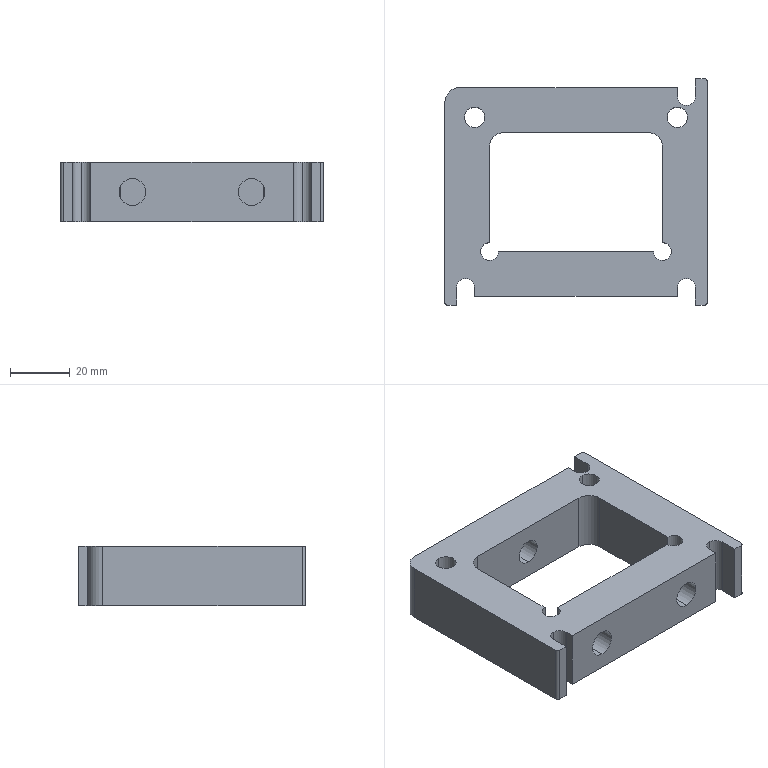Part | 1 solid | 45 faces | box 88 x 76 x 20 mm | volume 70626 mm3 | cylinder 26 | plane 19 | commonest cylinder face diameters 6 x10 6.8 x4 9 x4 2 x3 10 x3 8.5 x2
STEP:
#1=CARTESIAN_POINT('',(37.,29.,0.));
#2=VERTEX_POINT('',#1);
#3=CARTESIAN_POINT('',(34.,32.,0.));
#4=VERTEX_POINT('',#3);
#5=CARTESIAN_POINT('',(37.,32.,0.));
#6=DIRECTION('',(0.,0.,-1.));
#7=DIRECTION('',(0.,-1.,0.));
#8=AXIS2_PLACEMENT_3D('',#5,#6,#7);
#9=CIRCLE('',#8,3.);
#10=EDGE_CURVE('',#2,#4,#9,.T.);
#11=ORIENTED_EDGE('',*,*,#10,.F.);
#12=CARTESIAN_POINT('',(37.,29.,-20.));
#13=VERTEX_POINT('',#12);
#14=CARTESIAN_POINT('',(37.,29.,0.));
#15=DIRECTION('',(0.,0.,-1.));
#16=VECTOR('',#15,1000.);
#17=LINE('',#14,#16);
#18=EDGE_CURVE('',#2,#13,#17,.T.);
#19=ORIENTED_EDGE('',*,*,#18,.T.);
#20=CARTESIAN_POINT('',(34.,32.,-20.));
#21=VERTEX_POINT('',#20);
#22=CARTESIAN_POINT('',(37.,32.,-20.));
#23=DIRECTION('',(0.,0.,-1.));
#24=DIRECTION('',(0.,-1.,0.));
#25=AXIS2_PLACEMENT_3D('',#22,#23,#24);
#26=CIRCLE('',#25,3.);
#27=EDGE_CURVE('',#13,#21,#26,.T.);
#28=ORIENTED_EDGE('',*,*,#27,.T.);
#29=CARTESIAN_POINT('',(34.,32.,0.));
#30=DIRECTION('',(0.,0.,-1.));
#31=VECTOR('',#30,1000.);
#32=LINE('',#29,#31);
#33=EDGE_CURVE('',#4,#21,#32,.T.);
#34=ORIENTED_EDGE('',*,*,#33,.F.);
#35=EDGE_LOOP('',(#11,#19,#28,#34));
#36=FACE_BOUND('',#35,.T.);
#37=CARTESIAN_POINT('',(37.,32.,0.));
#38=DIRECTION('',(0.,0.,-1.));
#39=DIRECTION('',(0.,1.,0.));
#40=AXIS2_PLACEMENT_3D('',#37,#38,#39);
#41=CYLINDRICAL_SURFACE('',#40,3.);
#42=ADVANCED_FACE('',(#36),#41,.F.);
#43=CARTESIAN_POINT('',(-34.,21.6,0.));
#44=VERTEX_POINT('',#43);
#45=CARTESIAN_POINT('',(-34.,28.4,0.));
#46=VERTEX_POINT('',#45);
#47=CARTESIAN_POINT('',(-34.,25.,0.));
#48=DIRECTION('',(0.,0.,1.));
#49=DIRECTION('',(0.,1.,0.));
#50=AXIS2_PLACEMENT_3D('',#47,#48,#49);
#51=CIRCLE('',#50,3.4);
#52=EDGE_CURVE('',#44,#46,#51,.T.);
#53=ORIENTED_EDGE('',*,*,#52,.T.);
#54=CARTESIAN_POINT('',(-34.,28.4,-20.));
#55=VERTEX_POINT('',#54);
#56=CARTESIAN_POINT('',(-34.,28.4,-20.));
#57=DIRECTION('',(0.,0.,-1.));
#58=VECTOR('',#57,1000.);
#59=LINE('',#56,#58);
#60=EDGE_CURVE('',#55,#46,#59,.F.);
#61=ORIENTED_EDGE('',*,*,#60,.F.);
#62=CARTESIAN_POINT('',(-34.,21.6,-20.));
#63=VERTEX_POINT('',#62);
#64=CARTESIAN_POINT('',(-34.,25.,-20.));
#65=DIRECTION('',(0.,0.,-1.));
#66=DIRECTION('',(0.,-1.,0.));
#67=AXIS2_PLACEMENT_3D('',#64,#65,#66);
#68=CIRCLE('',#67,3.4);
#69=EDGE_CURVE('',#55,#63,#68,.T.);
#70=ORIENTED_EDGE('',*,*,#69,.T.);
#71=CARTESIAN_POINT('',(-34.,21.6,-20.));
#72=DIRECTION('',(0.,0.,-1.));
#73=VECTOR('',#72,1000.);
#74=LINE('',#71,#73);
#75=EDGE_CURVE('',#63,#44,#74,.F.);
#76=ORIENTED_EDGE('',*,*,#75,.T.);
#77=EDGE_LOOP('',(#53,#61,#70,#76));
#78=FACE_BOUND('',#77,.T.);
#79=CARTESIAN_POINT('',(-34.,25.,-20.));
#80=DIRECTION('',(0.,0.,-1.));
#81=DIRECTION('',(0.,1.,0.));
#82=AXIS2_PLACEMENT_3D('',#79,#80,#81);
#83=CYLINDRICAL_SURFACE('',#82,3.4);
#84=ADVANCED_FACE('',(#78),#83,.F.);
#85=CARTESIAN_POINT('',(34.,21.6,0.));
#86=VERTEX_POINT('',#85);
#87=CARTESIAN_POINT('',(34.,28.4,0.));
#88=VERTEX_POINT('',#87);
#89=CARTESIAN_POINT('',(34.,25.,0.));
#90=DIRECTION('',(0.,0.,1.));
#91=DIRECTION('',(0.,1.,0.));
#92=AXIS2_PLACEMENT_3D('',#89,#90,#91);
#93=CIRCLE('',#92,3.4);
#94=EDGE_CURVE('',#86,#88,#93,.T.);
#95=ORIENTED_EDGE('',*,*,#94,.T.);
#96=CARTESIAN_POINT('',(34.,28.4,-20.));
#97=VERTEX_POINT('',#96);
#98=CARTESIAN_POINT('',(34.,28.4,-20.));
#99=DIRECTION('',(0.,0.,-1.));
#100=VECTOR('',#99,1000.);
#101=LINE('',#98,#100);
#102=EDGE_CURVE('',#97,#88,#101,.F.);
#103=ORIENTED_EDGE('',*,*,#102,.F.);
#104=CARTESIAN_POINT('',(34.,21.6,-20.));
#105=VERTEX_POINT('',#104);
#106=CARTESIAN_POINT('',(34.,25.,-20.));
#107=DIRECTION('',(0.,0.,-1.));
#108=DIRECTION('',(0.,-1.,0.));
#109=AXIS2_PLACEMENT_3D('',#106,#107,#108);
#110=CIRCLE('',#109,3.4);
#111=EDGE_CURVE('',#97,#105,#110,.T.);
#112=ORIENTED_EDGE('',*,*,#111,.T.);
#113=CARTESIAN_POINT('',(34.,21.6,-20.));
#114=DIRECTION('',(0.,0.,-1.));
#115=VECTOR('',#114,1000.);
#116=LINE('',#113,#115);
#117=EDGE_CURVE('',#105,#86,#116,.F.);
#118=ORIENTED_EDGE('',*,*,#117,.T.);
#119=EDGE_LOOP('',(#95,#103,#112,#118));
#120=FACE_BOUND('',#119,.T.);
#121=CARTESIAN_POINT('',(34.,25.,-20.));
#122=DIRECTION('',(0.,0.,-1.));
#123=DIRECTION('',(0.,1.,0.));
#124=AXIS2_PLACEMENT_3D('',#121,#122,#123);
#125=CYLINDRICAL_SURFACE('',#124,3.4);
#126=ADVANCED_FACE('',(#120),#125,.F.);
#127=CARTESIAN_POINT('',(29.,-23.,0.));
#128=VERTEX_POINT('',#127);
#129=CARTESIAN_POINT('',(26.,-20.,0.));
#130=VERTEX_POINT('',#129);
#131=CARTESIAN_POINT('',(29.,-20.,0.));
#132=DIRECTION('',(0.,0.,-1.));
#133=DIRECTION('',(0.,-1.,0.));
#134=AXIS2_PLACEMENT_3D('',#131,#132,#133);
#135=CIRCLE('',#134,3.);
#136=EDGE_CURVE('',#128,#130,#135,.T.);
#137=ORIENTED_EDGE('',*,*,#136,.F.);
#138=CARTESIAN_POINT('',(29.,-23.,-20.));
#139=VERTEX_POINT('',#138);
#140=CARTESIAN_POINT('',(29.,-23.,0.));
#141=DIRECTION('',(0.,0.,-1.));
#142=VECTOR('',#141,1000.);
#143=LINE('',#140,#142);
#144=EDGE_CURVE('',#128,#139,#143,.T.);
#145=ORIENTED_EDGE('',*,*,#144,.T.);
#146=CARTESIAN_POINT('',(26.,-20.,-20.));
#147=VERTEX_POINT('',#146);
#148=CARTESIAN_POINT('',(29.,-20.,-20.));
#149=DIRECTION('',(0.,0.,-1.));
#150=DIRECTION('',(0.,-1.,0.));
#151=AXIS2_PLACEMENT_3D('',#148,#149,#150);
#152=CIRCLE('',#151,3.);
#153=EDGE_CURVE('',#139,#147,#152,.T.);
#154=ORIENTED_EDGE('',*,*,#153,.T.);
#155=CARTESIAN_POINT('',(26.,-20.,0.));
#156=DIRECTION('',(0.,0.,-1.));
#157=VECTOR('',#156,1000.);
#158=LINE('',#155,#157);
#159=EDGE_CURVE('',#130,#147,#158,.T.);
#160=ORIENTED_EDGE('',*,*,#159,.F.);
#161=EDGE_LOOP('',(#137,#145,#154,#160));
#162=FACE_BOUND('',#161,.T.);
#163=CARTESIAN_POINT('',(29.,-20.,0.));
#164=DIRECTION('',(0.,0.,-1.));
#165=DIRECTION('',(0.,1.,0.));
#166=AXIS2_PLACEMENT_3D('',#163,#164,#165);
#167=CYLINDRICAL_SURFACE('',#166,3.);
#168=ADVANCED_FACE('',(#162),#167,.F.);
#169=CARTESIAN_POINT('',(-29.,-23.,0.));
#170=VERTEX_POINT('',#169);
#171=CARTESIAN_POINT('',(-29.,-17.,0.));
#172=VERTEX_POINT('',#171);
#173=CARTESIAN_POINT('',(-29.,-20.,0.));
#174=DIRECTION('',(0.,0.,-1.));
#175=DIRECTION('',(0.,-1.,0.));
#176=AXIS2_PLACEMENT_3D('',#173,#174,#175);
#177=CIRCLE('',#176,3.);
#178=EDGE_CURVE('',#170,#172,#177,.T.);
#179=ORIENTED_EDGE('',*,*,#178,.F.);
#180=CARTESIAN_POINT('',(-29.,-23.,-20.));
#181=VERTEX_POINT('',#180);
#182=CARTESIAN_POINT('',(-29.,-23.,0.));
#183=DIRECTION('',(0.,0.,-1.));
#184=VECTOR('',#183,1000.);
#185=LINE('',#182,#184);
#186=EDGE_CURVE('',#170,#181,#185,.T.);
#187=ORIENTED_EDGE('',*,*,#186,.T.);
#188=CARTESIAN_POINT('',(-29.,-17.,-20.));
#189=VERTEX_POINT('',#188);
#190=CARTESIAN_POINT('',(-29.,-20.,-20.));
#191=DIRECTION('',(0.,0.,-1.));
#192=DIRECTION('',(0.,-1.,0.));
#193=AXIS2_PLACEMENT_3D('',#190,#191,#192);
#194=CIRCLE('',#193,3.);
#195=EDGE_CURVE('',#181,#189,#194,.T.);
#196=ORIENTED_EDGE('',*,*,#195,.T.);
#197=CARTESIAN_POINT('',(-29.,-17.,0.));
#198=DIRECTION('',(0.,0.,-1.));
#199=VECTOR('',#198,1000.);
#200=LINE('',#197,#199);
#201=EDGE_CURVE('',#172,#189,#200,.T.);
#202=ORIENTED_EDGE('',*,*,#201,.F.);
#203=EDGE_LOOP('',(#179,#187,#196,#202));
#204=FACE_BOUND('',#203,.T.);
#205=CARTESIAN_POINT('',(-29.,-20.,0.));
#206=DIRECTION('',(0.,0.,-1.));
#207=DIRECTION('',(0.,1.,0.));
#208=AXIS2_PLACEMENT_3D('',#205,#206,#207);
#209=CYLINDRICAL_SURFACE('',#208,3.);
#210=ADVANCED_FACE('',(#204),#209,.F.);
#211=CARTESIAN_POINT('',(20.,-20.,-5.5));
#212=VERTEX_POINT('',#211);
#213=CARTESIAN_POINT('',(20.,-20.,-14.5));
#214=VERTEX_POINT('',#213);
#215=CARTESIAN_POINT('',(20.,-20.,-10.));
#216=DIRECTION('',(0.,1.,0.));
#217=DIRECTION('',(0.,0.,1.));
#218=AXIS2_PLACEMENT_3D('',#215,#216,#217);
#219=CIRCLE('',#218,4.5);
#220=EDGE_CURVE('',#212,#214,#219,.T.);
#221=ORIENTED_EDGE('',*,*,#220,.T.);
#222=CARTESIAN_POINT('',(20.,-35.,-14.5));
#223=VERTEX_POINT('',#222);
#224=CARTESIAN_POINT('',(20.,15.,-14.5));
#225=DIRECTION('',(0.,-1.,0.));
#226=VECTOR('',#225,1000.);
#227=LINE('',#224,#226);
#228=EDGE_CURVE('',#223,#214,#227,.F.);
#229=ORIENTED_EDGE('',*,*,#228,.F.);
#230=CARTESIAN_POINT('',(20.,-35.,-5.5));
#231=VERTEX_POINT('',#230);
#232=CARTESIAN_POINT('',(20.,-35.,-10.));
#233=DIRECTION('',(0.,1.,0.));
#234=DIRECTION('',(0.,0.,1.));
#235=AXIS2_PLACEMENT_3D('',#232,#233,#234);
#236=CIRCLE('',#235,4.5);
#237=EDGE_CURVE('',#231,#223,#236,.T.);
#238=ORIENTED_EDGE('',*,*,#237,.F.);
#239=CARTESIAN_POINT('',(20.,15.,-5.5));
#240=DIRECTION('',(0.,-1.,0.));
#241=VECTOR('',#240,1000.);
#242=LINE('',#239,#241);
#243=EDGE_CURVE('',#231,#212,#242,.F.);
#244=ORIENTED_EDGE('',*,*,#243,.T.);
#245=EDGE_LOOP('',(#221,#229,#238,#244));
#246=FACE_BOUND('',#245,.T.);
#247=CARTESIAN_POINT('',(20.,15.,-10.));
#248=DIRECTION('',(0.,-1.,0.));
#249=DIRECTION('',(0.,0.,-1.));
#250=AXIS2_PLACEMENT_3D('',#247,#248,#249);
#251=CYLINDRICAL_SURFACE('',#250,4.5);
#252=ADVANCED_FACE('',(#246),#251,.F.);
#253=CARTESIAN_POINT('',(-20.,-20.,-14.5));
#254=VERTEX_POINT('',#253);
#255=CARTESIAN_POINT('',(-20.,-20.,-5.5));
#256=VERTEX_POINT('',#255);
#257=CARTESIAN_POINT('',(-20.,-20.,-10.));
#258=DIRECTION('',(0.,-1.,0.));
#259=DIRECTION('',(0.,0.,1.));
#260=AXIS2_PLACEMENT_3D('',#257,#258,#259);
#261=CIRCLE('',#260,4.5);
#262=EDGE_CURVE('',#254,#256,#261,.T.);
#263=ORIENTED_EDGE('',*,*,#262,.F.);
#264=CARTESIAN_POINT('',(-20.,-35.,-14.5));
#265=VERTEX_POINT('',#264);
#266=CARTESIAN_POINT('',(-20.,15.,-14.5));
#267=DIRECTION('',(0.,-1.,0.));
#268=VECTOR('',#267,1000.);
#269=LINE('',#266,#268);
#270=EDGE_CURVE('',#265,#254,#269,.F.);
#271=ORIENTED_EDGE('',*,*,#270,.F.);
#272=CARTESIAN_POINT('',(-20.,-35.,-5.5));
#273=VERTEX_POINT('',#272);
#274=CARTESIAN_POINT('',(-20.,-35.,-10.));
#275=DIRECTION('',(0.,-1.,0.));
#276=DIRECTION('',(0.,0.,1.));
#277=AXIS2_PLACEMENT_3D('',#274,#275,#276);
#278=CIRCLE('',#277,4.5);
#279=EDGE_CURVE('',#265,#273,#278,.T.);
#280=ORIENTED_EDGE('',*,*,#279,.T.);
#281=CARTESIAN_POINT('',(-20.,15.,-5.5));
#282=DIRECTION('',(0.,-1.,0.));
#283=VECTOR('',#282,1000.);
#284=LINE('',#281,#283);
#285=EDGE_CURVE('',#273,#256,#284,.F.);
#286=ORIENTED_EDGE('',*,*,#285,.T.);
#287=EDGE_LOOP('',(#263,#271,#280,#286));
#288=FACE_BOUND('',#287,.T.);
#289=CARTESIAN_POINT('',(-20.,15.,-10.));
#290=DIRECTION('',(0.,-1.,0.));
#291=DIRECTION('',(0.,0.,-1.));
#292=AXIS2_PLACEMENT_3D('',#289,#290,#291);
#293=CYLINDRICAL_SURFACE('',#292,4.5);
#294=ADVANCED_FACE('',(#288),#293,.F.);
#295=CARTESIAN_POINT('',(0.,20.,-5.75));
#296=VERTEX_POINT('',#295);
#297=CARTESIAN_POINT('',(0.,20.,-14.25));
#298=VERTEX_POINT('',#297);
#299=CARTESIAN_POINT('',(0.,20.,-10.));
#300=DIRECTION('',(0.,1.,0.));
#301=DIRECTION('',(0.,0.,-1.));
#302=AXIS2_PLACEMENT_3D('',#299,#300,#301);
#303=CIRCLE('',#302,4.25);
#304=EDGE_CURVE('',#296,#298,#303,.T.);
#305=ORIENTED_EDGE('',*,*,#304,.F.);
#306=CARTESIAN_POINT('',(0.,35.,-5.75));
#307=VERTEX_POINT('',#306);
#308=CARTESIAN_POINT('',(0.,35.,-5.75));
#309=DIRECTION('',(0.,1.,0.));
#310=VECTOR('',#309,1000.);
#311=LINE('',#308,#310);
#312=EDGE_CURVE('',#307,#296,#311,.F.);
#313=ORIENTED_EDGE('',*,*,#312,.F.);
#314=CARTESIAN_POINT('',(0.,35.,-14.25));
#315=VERTEX_POINT('',#314);
#316=CARTESIAN_POINT('',(0.,35.,-10.));
#317=DIRECTION('',(0.,1.,0.));
#318=DIRECTION('',(0.,0.,-1.));
#319=AXIS2_PLACEMENT_3D('',#316,#317,#318);
#320=CIRCLE('',#319,4.25);
#321=EDGE_CURVE('',#307,#315,#320,.T.);
#322=ORIENTED_EDGE('',*,*,#321,.T.);
#323=CARTESIAN_POINT('',(0.,35.,-14.25));
#324=DIRECTION('',(0.,1.,0.));
#325=VECTOR('',#324,1000.);
#326=LINE('',#323,#325);
#327=EDGE_CURVE('',#315,#298,#326,.F.);
#328=ORIENTED_EDGE('',*,*,#327,.T.);
#329=EDGE_LOOP('',(#305,#313,#322,#328));
#330=FACE_BOUND('',#329,.T.);
#331=CARTESIAN_POINT('',(0.,35.,-10.));
#332=DIRECTION('',(0.,1.,0.));
#333=DIRECTION('',(0.,0.,1.));
#334=AXIS2_PLACEMENT_3D('',#331,#332,#333);
#335=CYLINDRICAL_SURFACE('',#334,4.25);
#336=ADVANCED_FACE('',(#330),#335,.F.);
#337=CARTESIAN_POINT('',(-29.,15.,-20.));
#338=VERTEX_POINT('',#337);
#339=CARTESIAN_POINT('',(-29.,20.,-20.));
#340=DIRECTION('',(0.,1.,0.));
#341=VECTOR('',#340,1000.);
#342=LINE('',#339,#341);
#343=EDGE_CURVE('',#189,#338,#342,.T.);
#344=ORIENTED_EDGE('',*,*,#343,.F.);
#345=ORIENTED_EDGE('',*,*,#195,.F.);
#346=CARTESIAN_POINT('',(-26.,-20.,-20.));
#347=VERTEX_POINT('',#346);
#348=CARTESIAN_POINT('',(-29.,-20.,-20.));
#349=DIRECTION('',(0.,0.,-1.));
#350=DIRECTION('',(0.,-1.,0.));
#351=AXIS2_PLACEMENT_3D('',#348,#349,#350);
#352=CIRCLE('',#351,3.);
#353=EDGE_CURVE('',#347,#181,#352,.T.);
#354=ORIENTED_EDGE('',*,*,#353,.F.);
#355=CARTESIAN_POINT('',(29.,-20.,-20.));
#356=DIRECTION('',(-1.,0.,0.));
#357=VECTOR('',#356,1000.);
#358=LINE('',#355,#357);
#359=EDGE_CURVE('',#147,#347,#358,.T.);
#360=ORIENTED_EDGE('',*,*,#359,.F.);
#361=ORIENTED_EDGE('',*,*,#153,.F.);
#362=CARTESIAN_POINT('',(29.,-17.,-20.));
#363=VERTEX_POINT('',#362);
#364=CARTESIAN_POINT('',(29.,-20.,-20.));
#365=DIRECTION('',(0.,0.,-1.));
#366=DIRECTION('',(0.,-1.,0.));
#367=AXIS2_PLACEMENT_3D('',#364,#365,#366);
#368=CIRCLE('',#367,3.);
#369=EDGE_CURVE('',#363,#139,#368,.T.);
#370=ORIENTED_EDGE('',*,*,#369,.F.);
#371=CARTESIAN_POINT('',(29.,15.,-20.));
#372=VERTEX_POINT('',#371);
#373=CARTESIAN_POINT('',(29.,20.,-20.));
#374=DIRECTION('',(0.,-1.,0.));
#375=VECTOR('',#374,1000.);
#376=LINE('',#373,#375);
#377=EDGE_CURVE('',#372,#363,#376,.T.);
#378=ORIENTED_EDGE('',*,*,#377,.F.);
#379=CARTESIAN_POINT('',(24.,20.,-20.));
#380=VERTEX_POINT('',#379);
#381=CARTESIAN_POINT('',(24.,15.,-20.));
#382=DIRECTION('',(0.,0.,1.));
#383=DIRECTION('',(0.,1.,0.));
#384=AXIS2_PLACEMENT_3D('',#381,#382,#383);
#385=CIRCLE('',#384,5.);
#386=EDGE_CURVE('',#372,#380,#385,.T.);
#387=ORIENTED_EDGE('',*,*,#386,.T.);
#388=CARTESIAN_POINT('',(-24.,20.,-20.));
#389=VERTEX_POINT('',#388);
#390=CARTESIAN_POINT('',(29.,20.,-20.));
#391=DIRECTION('',(1.,0.,0.));
#392=VECTOR('',#391,1000.);
#393=LINE('',#390,#392);
#394=EDGE_CURVE('',#389,#380,#393,.T.);
#395=ORIENTED_EDGE('',*,*,#394,.F.);
#396=CARTESIAN_POINT('',(-24.,15.,-20.));
#397=DIRECTION('',(0.,0.,1.));
#398=DIRECTION('',(0.,1.,0.));
#399=AXIS2_PLACEMENT_3D('',#396,#397,#398);
#400=CIRCLE('',#399,5.);
#401=EDGE_CURVE('',#389,#338,#400,.T.);
#402=ORIENTED_EDGE('',*,*,#401,.T.);
#403=EDGE_LOOP('',(#344,#345,#354,#360,#361,#370,#378,#387,#395,#402));
#404=FACE_BOUND('',#403,.T.);
#405=CARTESIAN_POINT('',(34.,25.,-20.));
#406=DIRECTION('',(0.,0.,-1.));
#407=DIRECTION('',(0.,-1.,0.));
#408=AXIS2_PLACEMENT_3D('',#405,#406,#407);
#409=CIRCLE('',#408,3.4);
#410=EDGE_CURVE('',#105,#97,#409,.T.);
#411=ORIENTED_EDGE('',*,*,#410,.F.);
#412=ORIENTED_EDGE('',*,*,#111,.F.);
#413=EDGE_LOOP('',(#411,#412));
#414=FACE_BOUND('',#413,.T.);
#415=CARTESIAN_POINT('',(-34.,25.,-20.));
#416=DIRECTION('',(0.,0.,-1.));
#417=DIRECTION('',(0.,-1.,0.));
#418=AXIS2_PLACEMENT_3D('',#415,#416,#417);
#419=CIRCLE('',#418,3.4);
#420=EDGE_CURVE('',#63,#55,#419,.T.);
#421=ORIENTED_EDGE('',*,*,#420,.F.);
#422=ORIENTED_EDGE('',*,*,#69,.F.);
#423=EDGE_LOOP('',(#421,#422));
#424=FACE_BOUND('',#423,.T.);
#425=CARTESIAN_POINT('',(-40.,-38.,-20.));
#426=VERTEX_POINT('',#425);
#427=CARTESIAN_POINT('',(-43.,-38.,-20.));
#428=VERTEX_POINT('',#427);
#429=CARTESIAN_POINT('',(44.,-38.,-20.));
#430=DIRECTION('',(-1.,0.,0.));
#431=VECTOR('',#430,1000.);
#432=LINE('',#429,#431);
#433=EDGE_CURVE('',#426,#428,#432,.T.);
#434=ORIENTED_EDGE('',*,*,#433,.T.);
#435=CARTESIAN_POINT('',(-44.,-37.,-20.));
#436=VERTEX_POINT('',#435);
#437=CARTESIAN_POINT('',(-43.,-37.,-20.));
#438=DIRECTION('',(0.,0.,-1.));
#439=DIRECTION('',(0.,1.,0.));
#440=AXIS2_PLACEMENT_3D('',#437,#438,#439);
#441=CIRCLE('',#440,1.);
#442=EDGE_CURVE('',#428,#436,#441,.T.);
#443=ORIENTED_EDGE('',*,*,#442,.T.);
#444=CARTESIAN_POINT('',(-44.,30.,-20.));
#445=VERTEX_POINT('',#444);
#446=CARTESIAN_POINT('',(-44.,38.,-20.));
#447=DIRECTION('',(0.,1.,0.));
#448=VECTOR('',#447,1000.);
#449=LINE('',#446,#448);
#450=EDGE_CURVE('',#436,#445,#449,.T.);
#451=ORIENTED_EDGE('',*,*,#450,.T.);
#452=CARTESIAN_POINT('',(-39.,35.,-20.));
#453=VERTEX_POINT('',#452);
#454=CARTESIAN_POINT('',(-39.,30.,-20.));
#455=DIRECTION('',(0.,0.,-1.));
#456=DIRECTION('',(0.,1.,0.));
#457=AXIS2_PLACEMENT_3D('',#454,#455,#456);
#458=CIRCLE('',#457,5.);
#459=EDGE_CURVE('',#445,#453,#458,.T.);
#460=ORIENTED_EDGE('',*,*,#459,.T.);
#461=CARTESIAN_POINT('',(34.,35.,-20.));
#462=VERTEX_POINT('',#461);
#463=CARTESIAN_POINT('',(-44.,35.,-20.));
#464=DIRECTION('',(-1.,0.,0.));
#465=VECTOR('',#464,1000.);
#466=LINE('',#463,#465);
#467=EDGE_CURVE('',#462,#453,#466,.T.);
#468=ORIENTED_EDGE('',*,*,#467,.F.);
#469=CARTESIAN_POINT('',(34.,38.,-20.));
#470=DIRECTION('',(0.,1.,0.));
#471=VECTOR('',#470,1000.);
#472=LINE('',#469,#471);
#473=EDGE_CURVE('',#21,#462,#472,.T.);
#474=ORIENTED_EDGE('',*,*,#473,.F.);
#475=ORIENTED_EDGE('',*,*,#27,.F.);
#476=CARTESIAN_POINT('',(40.,32.,-20.));
#477=VERTEX_POINT('',#476);
#478=CARTESIAN_POINT('',(37.,32.,-20.));
#479=DIRECTION('',(0.,0.,-1.));
#480=DIRECTION('',(0.,-1.,0.));
#481=AXIS2_PLACEMENT_3D('',#478,#479,#480);
#482=CIRCLE('',#481,3.);
#483=EDGE_CURVE('',#477,#13,#482,.T.);
#484=ORIENTED_EDGE('',*,*,#483,.F.);
#485=CARTESIAN_POINT('',(40.,38.,-20.));
#486=VERTEX_POINT('',#485);
#487=CARTESIAN_POINT('',(40.,38.,-20.));
#488=DIRECTION('',(0.,-1.,0.));
#489=VECTOR('',#488,1000.);
#490=LINE('',#487,#489);
#491=EDGE_CURVE('',#486,#477,#490,.T.);
#492=ORIENTED_EDGE('',*,*,#491,.F.);
#493=CARTESIAN_POINT('',(43.,38.,-20.));
#494=VERTEX_POINT('',#493);
#495=CARTESIAN_POINT('',(44.,38.,-20.));
#496=DIRECTION('',(1.,0.,0.));
#497=VECTOR('',#496,1000.);
#498=LINE('',#495,#497);
#499=EDGE_CURVE('',#486,#494,#498,.T.);
#500=ORIENTED_EDGE('',*,*,#499,.T.);
#501=CARTESIAN_POINT('',(44.,37.,-20.));
#502=VERTEX_POINT('',#501);
#503=CARTESIAN_POINT('',(43.,37.,-20.));
#504=DIRECTION('',(0.,0.,-1.));
#505=DIRECTION('',(0.,1.,0.));
#506=AXIS2_PLACEMENT_3D('',#503,#504,#505);
#507=CIRCLE('',#506,1.);
#508=EDGE_CURVE('',#494,#502,#507,.T.);
#509=ORIENTED_EDGE('',*,*,#508,.T.);
#510=CARTESIAN_POINT('',(44.,-37.,-20.));
#511=VERTEX_POINT('',#510);
#512=CARTESIAN_POINT('',(44.,38.,-20.));
#513=DIRECTION('',(0.,-1.,0.));
#514=VECTOR('',#513,1000.);
#515=LINE('',#512,#514);
#516=EDGE_CURVE('',#502,#511,#515,.T.);
#517=ORIENTED_EDGE('',*,*,#516,.T.);
#518=CARTESIAN_POINT('',(43.,-38.,-20.));
#519=VERTEX_POINT('',#518);
#520=CARTESIAN_POINT('',(43.,-37.,-20.));
#521=DIRECTION('',(0.,0.,-1.));
#522=DIRECTION('',(0.,1.,0.));
#523=AXIS2_PLACEMENT_3D('',#520,#521,#522);
#524=CIRCLE('',#523,1.);
#525=EDGE_CURVE('',#511,#519,#524,.T.);
#526=ORIENTED_EDGE('',*,*,#525,.T.);
#527=CARTESIAN_POINT('',(40.,-38.,-20.));
#528=VERTEX_POINT('',#527);
#529=CARTESIAN_POINT('',(44.,-38.,-20.));
#530=DIRECTION('',(-1.,0.,0.));
#531=VECTOR('',#530,1000.);
#532=LINE('',#529,#531);
#533=EDGE_CURVE('',#519,#528,#532,.T.);
#534=ORIENTED_EDGE('',*,*,#533,.T.);
#535=CARTESIAN_POINT('',(40.,-32.,-20.));
#536=VERTEX_POINT('',#535);
#537=CARTESIAN_POINT('',(40.,-41.,-20.));
#538=DIRECTION('',(0.,-1.,0.));
#539=VECTOR('',#538,1000.);
#540=LINE('',#537,#539);
#541=EDGE_CURVE('',#536,#528,#540,.T.);
#542=ORIENTED_EDGE('',*,*,#541,.F.);
#543=CARTESIAN_POINT('',(37.,-29.,-20.));
#544=VERTEX_POINT('',#543);
#545=CARTESIAN_POINT('',(37.,-32.,-20.));
#546=DIRECTION('',(0.,0.,1.));
#547=DIRECTION('',(0.,1.,0.));
#548=AXIS2_PLACEMENT_3D('',#545,#546,#547);
#549=CIRCLE('',#548,3.);
#550=EDGE_CURVE('',#536,#544,#549,.T.);
#551=ORIENTED_EDGE('',*,*,#550,.T.);
#552=CARTESIAN_POINT('',(34.,-32.,-20.));
#553=VERTEX_POINT('',#552);
#554=CARTESIAN_POINT('',(37.,-32.,-20.));
#555=DIRECTION('',(0.,0.,1.));
#556=DIRECTION('',(0.,1.,0.));
#557=AXIS2_PLACEMENT_3D('',#554,#555,#556);
#558=CIRCLE('',#557,3.);
#559=EDGE_CURVE('',#544,#553,#558,.T.);
#560=ORIENTED_EDGE('',*,*,#559,.T.);
#561=CARTESIAN_POINT('',(34.,-35.,-20.));
#562=VERTEX_POINT('',#561);
#563=CARTESIAN_POINT('',(34.,-35.,-20.));
#564=DIRECTION('',(0.,-1.,0.));
#565=VECTOR('',#564,1000.);
#566=LINE('',#563,#565);
#567=EDGE_CURVE('',#553,#562,#566,.T.);
#568=ORIENTED_EDGE('',*,*,#567,.T.);
#569=CARTESIAN_POINT('',(-34.,-35.,-20.));
#570=VERTEX_POINT('',#569);
#571=CARTESIAN_POINT('',(40.,-35.,-20.));
#572=DIRECTION('',(1.,0.,0.));
#573=VECTOR('',#572,1000.);
#574=LINE('',#571,#573);
#575=EDGE_CURVE('',#570,#562,#574,.T.);
#576=ORIENTED_EDGE('',*,*,#575,.F.);
#577=CARTESIAN_POINT('',(-34.,-32.,-20.));
#578=VERTEX_POINT('',#577);
#579=CARTESIAN_POINT('',(-34.,-35.,-20.));
#580=DIRECTION('',(0.,-1.,0.));
#581=VECTOR('',#580,1000.);
#582=LINE('',#579,#581);
#583=EDGE_CURVE('',#578,#570,#582,.T.);
#584=ORIENTED_EDGE('',*,*,#583,.F.);
#585=CARTESIAN_POINT('',(-37.,-29.,-20.));
#586=VERTEX_POINT('',#585);
#587=CARTESIAN_POINT('',(-37.,-32.,-20.));
#588=DIRECTION('',(0.,0.,1.));
#589=DIRECTION('',(0.,1.,0.));
#590=AXIS2_PLACEMENT_3D('',#587,#588,#589);
#591=CIRCLE('',#590,3.);
#592=EDGE_CURVE('',#578,#586,#591,.T.);
#593=ORIENTED_EDGE('',*,*,#592,.T.);
#594=CARTESIAN_POINT('',(-40.,-32.,-20.));
#595=VERTEX_POINT('',#594);
#596=CARTESIAN_POINT('',(-37.,-32.,-20.));
#597=DIRECTION('',(0.,0.,1.));
#598=DIRECTION('',(0.,1.,0.));
#599=AXIS2_PLACEMENT_3D('',#596,#597,#598);
#600=CIRCLE('',#599,3.);
#601=EDGE_CURVE('',#586,#595,#600,.T.);
#602=ORIENTED_EDGE('',*,*,#601,.T.);
#603=CARTESIAN_POINT('',(-40.,-41.,-20.));
#604=DIRECTION('',(0.,1.,0.));
#605=VECTOR('',#604,1000.);
#606=LINE('',#603,#605);
#607=EDGE_CURVE('',#426,#595,#606,.T.);
#608=ORIENTED_EDGE('',*,*,#607,.F.);
#609=EDGE_LOOP('',(#434,#443,#451,#460,#468,#474,#475,#484,#492,#500,#509,#517,#526,#534,#542,#551,#560,#568,#576,#584,#593,#602,#608));
#610=FACE_BOUND('',#609,.T.);
#611=CARTESIAN_POINT('',(0.,0.,-20.));
#612=DIRECTION('',(0.,0.,1.));
#613=DIRECTION('',(0.,-1.,0.));
#614=AXIS2_PLACEMENT_3D('',#611,#612,#613);
#615=PLANE('',#614);
#616=ADVANCED_FACE('',(#404,#414,#424,#610),#615,.F.);
#617=CARTESIAN_POINT('',(-44.,-37.,0.));
#618=VERTEX_POINT('',#617);
#619=CARTESIAN_POINT('',(-44.,30.,0.));
#620=VERTEX_POINT('',#619);
#621=CARTESIAN_POINT('',(-44.,38.,0.));
#622=DIRECTION('',(0.,1.,0.));
#623=VECTOR('',#622,1000.);
#624=LINE('',#621,#623);
#625=EDGE_CURVE('',#618,#620,#624,.T.);
#626=ORIENTED_EDGE('',*,*,#625,.F.);
#627=CARTESIAN_POINT('',(-43.,-38.,0.));
#628=VERTEX_POINT('',#627);
#629=CARTESIAN_POINT('',(-43.,-37.,0.));
#630=DIRECTION('',(0.,0.,1.));
#631=DIRECTION('',(0.,1.,0.));
#632=AXIS2_PLACEMENT_3D('',#629,#630,#631);
#633=CIRCLE('',#632,1.);
#634=EDGE_CURVE('',#618,#628,#633,.T.);
#635=ORIENTED_EDGE('',*,*,#634,.T.);
#636=CARTESIAN_POINT('',(-40.,-38.,0.));
#637=VERTEX_POINT('',#636);
#638=CARTESIAN_POINT('',(44.,-38.,0.));
#639=DIRECTION('',(-1.,0.,0.));
#640=VECTOR('',#639,1000.);
#641=LINE('',#638,#640);
#642=EDGE_CURVE('',#637,#628,#641,.T.);
#643=ORIENTED_EDGE('',*,*,#642,.F.);
#644=CARTESIAN_POINT('',(-40.,-32.,0.));
#645=VERTEX_POINT('',#644);
#646=CARTESIAN_POINT('',(-40.,0.,0.));
#647=DIRECTION('',(0.,-1.,0.));
#648=VECTOR('',#647,1000.);
#649=LINE('',#646,#648);
#650=EDGE_CURVE('',#645,#637,#649,.T.);
#651=ORIENTED_EDGE('',*,*,#650,.F.);
#652=CARTESIAN_POINT('',(-37.,-29.,0.));
#653=VERTEX_POINT('',#652);
#654=CARTESIAN_POINT('',(-37.,-32.,0.));
#655=DIRECTION('',(0.,0.,-1.));
#656=DIRECTION('',(0.,1.,0.));
#657=AXIS2_PLACEMENT_3D('',#654,#655,#656);
#658=CIRCLE('',#657,3.);
#659=EDGE_CURVE('',#645,#653,#658,.T.);
#660=ORIENTED_EDGE('',*,*,#659,.T.);
#661=CARTESIAN_POINT('',(-34.,-32.,0.));
#662=VERTEX_POINT('',#661);
#663=CARTESIAN_POINT('',(-37.,-32.,0.));
#664=DIRECTION('',(0.,0.,-1.));
#665=DIRECTION('',(0.,1.,0.));
#666=AXIS2_PLACEMENT_3D('',#663,#664,#665);
#667=CIRCLE('',#666,3.);
#668=EDGE_CURVE('',#653,#662,#667,.T.);
#669=ORIENTED_EDGE('',*,*,#668,.T.);
#670=CARTESIAN_POINT('',(-34.,-35.,0.));
#671=VERTEX_POINT('',#670);
#672=CARTESIAN_POINT('',(-34.,-35.,0.));
#673=DIRECTION('',(0.,-1.,0.));
#674=VECTOR('',#673,1000.);
#675=LINE('',#672,#674);
#676=EDGE_CURVE('',#662,#671,#675,.T.);
#677=ORIENTED_EDGE('',*,*,#676,.T.);
#678=CARTESIAN_POINT('',(34.,-35.,0.));
#679=VERTEX_POINT('',#678);
#680=CARTESIAN_POINT('',(40.,-35.,0.));
#681=DIRECTION('',(1.,0.,0.));
#682=VECTOR('',#681,1000.);
#683=LINE('',#680,#682);
#684=EDGE_CURVE('',#671,#679,#683,.T.);
#685=ORIENTED_EDGE('',*,*,#684,.T.);
#686=CARTESIAN_POINT('',(34.,-32.,0.));
#687=VERTEX_POINT('',#686);
#688=CARTESIAN_POINT('',(34.,-35.,0.));
#689=DIRECTION('',(0.,-1.,0.));
#690=VECTOR('',#689,1000.);
#691=LINE('',#688,#690);
#692=EDGE_CURVE('',#687,#679,#691,.T.);
#693=ORIENTED_EDGE('',*,*,#692,.F.);
#694=CARTESIAN_POINT('',(37.,-29.,0.));
#695=VERTEX_POINT('',#694);
#696=CARTESIAN_POINT('',(37.,-32.,0.));
#697=DIRECTION('',(0.,0.,-1.));
#698=DIRECTION('',(0.,1.,0.));
#699=AXIS2_PLACEMENT_3D('',#696,#697,#698);
#700=CIRCLE('',#699,3.);
#701=EDGE_CURVE('',#687,#695,#700,.T.);
#702=ORIENTED_EDGE('',*,*,#701,.T.);
#703=CARTESIAN_POINT('',(40.,-32.,0.));
#704=VERTEX_POINT('',#703);
#705=CARTESIAN_POINT('',(37.,-32.,0.));
#706=DIRECTION('',(0.,0.,-1.));
#707=DIRECTION('',(0.,1.,0.));
#708=AXIS2_PLACEMENT_3D('',#705,#706,#707);
#709=CIRCLE('',#708,3.);
#710=EDGE_CURVE('',#695,#704,#709,.T.);
#711=ORIENTED_EDGE('',*,*,#710,.T.);
#712=CARTESIAN_POINT('',(40.,-38.,0.));
#713=VERTEX_POINT('',#712);
#714=CARTESIAN_POINT('',(40.,-41.,0.));
#715=DIRECTION('',(0.,-1.,0.));
#716=VECTOR('',#715,1000.);
#717=LINE('',#714,#716);
#718=EDGE_CURVE('',#704,#713,#717,.T.);
#719=ORIENTED_EDGE('',*,*,#718,.T.);
#720=CARTESIAN_POINT('',(43.,-38.,0.));
#721=VERTEX_POINT('',#720);
#722=CARTESIAN_POINT('',(44.,-38.,0.));
#723=DIRECTION('',(-1.,0.,0.));
#724=VECTOR('',#723,1000.);
#725=LINE('',#722,#724);
#726=EDGE_CURVE('',#721,#713,#725,.T.);
#727=ORIENTED_EDGE('',*,*,#726,.F.);
#728=CARTESIAN_POINT('',(44.,-37.,0.));
#729=VERTEX_POINT('',#728);
#730=CARTESIAN_POINT('',(43.,-37.,0.));
#731=DIRECTION('',(0.,0.,1.));
#732=DIRECTION('',(0.,1.,0.));
#733=AXIS2_PLACEMENT_3D('',#730,#731,#732);
#734=CIRCLE('',#733,1.);
#735=EDGE_CURVE('',#721,#729,#734,.T.);
#736=ORIENTED_EDGE('',*,*,#735,.T.);
#737=CARTESIAN_POINT('',(44.,37.,0.));
#738=VERTEX_POINT('',#737);
#739=CARTESIAN_POINT('',(44.,38.,0.));
#740=DIRECTION('',(0.,-1.,0.));
#741=VECTOR('',#740,1000.);
#742=LINE('',#739,#741);
#743=EDGE_CURVE('',#738,#729,#742,.T.);
#744=ORIENTED_EDGE('',*,*,#743,.F.);
#745=CARTESIAN_POINT('',(43.,38.,0.));
#746=VERTEX_POINT('',#745);
#747=CARTESIAN_POINT('',(43.,37.,0.));
#748=DIRECTION('',(0.,0.,1.));
#749=DIRECTION('',(0.,1.,0.));
#750=AXIS2_PLACEMENT_3D('',#747,#748,#749);
#751=CIRCLE('',#750,1.);
#752=EDGE_CURVE('',#738,#746,#751,.T.);
#753=ORIENTED_EDGE('',*,*,#752,.T.);
#754=CARTESIAN_POINT('',(40.,38.,0.));
#755=VERTEX_POINT('',#754);
#756=CARTESIAN_POINT('',(44.,38.,0.));
#757=DIRECTION('',(1.,0.,0.));
#758=VECTOR('',#757,1000.);
#759=LINE('',#756,#758);
#760=EDGE_CURVE('',#755,#746,#759,.T.);
#761=ORIENTED_EDGE('',*,*,#760,.F.);
#762=CARTESIAN_POINT('',(40.,32.,0.));
#763=VERTEX_POINT('',#762);
#764=CARTESIAN_POINT('',(40.,38.,0.));
#765=DIRECTION('',(0.,-1.,0.));
#766=VECTOR('',#765,1000.);
#767=LINE('',#764,#766);
#768=EDGE_CURVE('',#755,#763,#767,.T.);
#769=ORIENTED_EDGE('',*,*,#768,.T.);
#770=CARTESIAN_POINT('',(37.,32.,0.));
#771=DIRECTION('',(0.,0.,-1.));
#772=DIRECTION('',(0.,-1.,0.));
#773=AXIS2_PLACEMENT_3D('',#770,#771,#772);
#774=CIRCLE('',#773,3.);
#775=EDGE_CURVE('',#763,#2,#774,.T.);
#776=ORIENTED_EDGE('',*,*,#775,.T.);
#777=ORIENTED_EDGE('',*,*,#10,.T.);
#778=CARTESIAN_POINT('',(34.,35.,0.));
#779=VERTEX_POINT('',#778);
#780=CARTESIAN_POINT('',(34.,38.,0.));
#781=DIRECTION('',(0.,1.,0.));
#782=VECTOR('',#781,1000.);
#783=LINE('',#780,#782);
#784=EDGE_CURVE('',#4,#779,#783,.T.);
#785=ORIENTED_EDGE('',*,*,#784,.T.);
#786=CARTESIAN_POINT('',(-39.,35.,0.));
#787=VERTEX_POINT('',#786);
#788=CARTESIAN_POINT('',(-44.,35.,0.));
#789=DIRECTION('',(-1.,0.,0.));
#790=VECTOR('',#789,1000.);
#791=LINE('',#788,#790);
#792=EDGE_CURVE('',#779,#787,#791,.T.);
#793=ORIENTED_EDGE('',*,*,#792,.T.);
#794=CARTESIAN_POINT('',(-39.,30.,0.));
#795=DIRECTION('',(0.,0.,1.));
#796=DIRECTION('',(0.,1.,0.));
#797=AXIS2_PLACEMENT_3D('',#794,#795,#796);
#798=CIRCLE('',#797,5.);
#799=EDGE_CURVE('',#787,#620,#798,.T.);
#800=ORIENTED_EDGE('',*,*,#799,.T.);
#801=EDGE_LOOP('',(#626,#635,#643,#651,#660,#669,#677,#685,#693,#702,#711,#719,#727,#736,#744,#753,#761,#769,#776,#777,#785,#793,#800));
#802=FACE_BOUND('',#801,.T.);
#803=ORIENTED_EDGE('',*,*,#52,.F.);
#804=CARTESIAN_POINT('',(-34.,25.,0.));
#805=DIRECTION('',(0.,0.,1.));
#806=DIRECTION('',(0.,1.,0.));
#807=AXIS2_PLACEMENT_3D('',#804,#805,#806);
#808=CIRCLE('',#807,3.4);
#809=EDGE_CURVE('',#46,#44,#808,.T.);
#810=ORIENTED_EDGE('',*,*,#809,.F.);
#811=EDGE_LOOP('',(#803,#810));
#812=FACE_BOUND('',#811,.T.);
#813=ORIENTED_EDGE('',*,*,#94,.F.);
#814=CARTESIAN_POINT('',(34.,25.,0.));
#815=DIRECTION('',(0.,0.,1.));
#816=DIRECTION('',(0.,1.,0.));
#817=AXIS2_PLACEMENT_3D('',#814,#815,#816);
#818=CIRCLE('',#817,3.4);
#819=EDGE_CURVE('',#88,#86,#818,.T.);
#820=ORIENTED_EDGE('',*,*,#819,.F.);
#821=EDGE_LOOP('',(#813,#820));
#822=FACE_BOUND('',#821,.T.);
#823=CARTESIAN_POINT('',(-26.,-20.,0.));
#824=VERTEX_POINT('',#823);
#825=CARTESIAN_POINT('',(-29.,-20.,0.));
#826=DIRECTION('',(0.,0.,-1.));
#827=DIRECTION('',(0.,-1.,0.));
#828=AXIS2_PLACEMENT_3D('',#825,#826,#827);
#829=CIRCLE('',#828,3.);
#830=EDGE_CURVE('',#824,#170,#829,.T.);
#831=ORIENTED_EDGE('',*,*,#830,.T.);
#832=ORIENTED_EDGE('',*,*,#178,.T.);
#833=CARTESIAN_POINT('',(-29.,15.,0.));
#834=VERTEX_POINT('',#833);
#835=CARTESIAN_POINT('',(-29.,20.,0.));
#836=DIRECTION('',(0.,1.,0.));
#837=VECTOR('',#836,1000.);
#838=LINE('',#835,#837);
#839=EDGE_CURVE('',#172,#834,#838,.T.);
#840=ORIENTED_EDGE('',*,*,#839,.T.);
#841=CARTESIAN_POINT('',(-24.,20.,0.));
#842=VERTEX_POINT('',#841);
#843=CARTESIAN_POINT('',(-24.,15.,0.));
#844=DIRECTION('',(0.,0.,-1.));
#845=DIRECTION('',(0.,1.,0.));
#846=AXIS2_PLACEMENT_3D('',#843,#844,#845);
#847=CIRCLE('',#846,5.);
#848=EDGE_CURVE('',#834,#842,#847,.T.);
#849=ORIENTED_EDGE('',*,*,#848,.T.);
#850=CARTESIAN_POINT('',(24.,20.,0.));
#851=VERTEX_POINT('',#850);
#852=CARTESIAN_POINT('',(29.,20.,0.));
#853=DIRECTION('',(1.,0.,0.));
#854=VECTOR('',#853,1000.);
#855=LINE('',#852,#854);
#856=EDGE_CURVE('',#842,#851,#855,.T.);
#857=ORIENTED_EDGE('',*,*,#856,.T.);
#858=CARTESIAN_POINT('',(29.,15.,0.));
#859=VERTEX_POINT('',#858);
#860=CARTESIAN_POINT('',(24.,15.,0.));
#861=DIRECTION('',(0.,0.,-1.));
#862=DIRECTION('',(0.,1.,0.));
#863=AXIS2_PLACEMENT_3D('',#860,#861,#862);
#864=CIRCLE('',#863,5.);
#865=EDGE_CURVE('',#851,#859,#864,.T.);
#866=ORIENTED_EDGE('',*,*,#865,.T.);
#867=CARTESIAN_POINT('',(29.,-17.,0.));
#868=VERTEX_POINT('',#867);
#869=CARTESIAN_POINT('',(29.,20.,0.));
#870=DIRECTION('',(0.,-1.,0.));
#871=VECTOR('',#870,1000.);
#872=LINE('',#869,#871);
#873=EDGE_CURVE('',#859,#868,#872,.T.);
#874=ORIENTED_EDGE('',*,*,#873,.T.);
#875=CARTESIAN_POINT('',(29.,-20.,0.));
#876=DIRECTION('',(0.,0.,-1.));
#877=DIRECTION('',(0.,-1.,0.));
#878=AXIS2_PLACEMENT_3D('',#875,#876,#877);
#879=CIRCLE('',#878,3.);
#880=EDGE_CURVE('',#868,#128,#879,.T.);
#881=ORIENTED_EDGE('',*,*,#880,.T.);
#882=ORIENTED_EDGE('',*,*,#136,.T.);
#883=CARTESIAN_POINT('',(29.,-20.,0.));
#884=DIRECTION('',(-1.,0.,0.));
#885=VECTOR('',#884,1000.);
#886=LINE('',#883,#885);
#887=EDGE_CURVE('',#130,#824,#886,.T.);
#888=ORIENTED_EDGE('',*,*,#887,.T.);
#889=EDGE_LOOP('',(#831,#832,#840,#849,#857,#866,#874,#881,#882,#888));
#890=FACE_BOUND('',#889,.T.);
#891=CARTESIAN_POINT('',(0.,0.,0.));
#892=DIRECTION('',(0.,0.,1.));
#893=DIRECTION('',(0.,-1.,0.));
#894=AXIS2_PLACEMENT_3D('',#891,#892,#893);
#895=PLANE('',#894);
#896=ADVANCED_FACE('',(#802,#812,#822,#890),#895,.T.);
#897=CARTESIAN_POINT('',(-20.,-35.,-10.));
#898=DIRECTION('',(0.,-1.,0.));
#899=DIRECTION('',(0.,0.,1.));
#900=AXIS2_PLACEMENT_3D('',#897,#898,#899);
#901=CIRCLE('',#900,4.5);
#902=EDGE_CURVE('',#273,#265,#901,.T.);
#903=ORIENTED_EDGE('',*,*,#902,.F.);
#904=ORIENTED_EDGE('',*,*,#279,.F.);
#905=EDGE_LOOP('',(#903,#904));
#906=FACE_BOUND('',#905,.T.);
#907=ORIENTED_EDGE('',*,*,#237,.T.);
#908=CARTESIAN_POINT('',(20.,-35.,-10.));
#909=DIRECTION('',(0.,1.,0.));
#910=DIRECTION('',(0.,0.,1.));
#911=AXIS2_PLACEMENT_3D('',#908,#909,#910);
#912=CIRCLE('',#911,4.5);
#913=EDGE_CURVE('',#223,#231,#912,.T.);
#914=ORIENTED_EDGE('',*,*,#913,.T.);
#915=EDGE_LOOP('',(#907,#914));
#916=FACE_BOUND('',#915,.T.);
#917=CARTESIAN_POINT('',(34.,-35.,0.));
#918=DIRECTION('',(0.,0.,-1.));
#919=VECTOR('',#918,1000.);
#920=LINE('',#917,#919);
#921=EDGE_CURVE('',#679,#562,#920,.T.);
#922=ORIENTED_EDGE('',*,*,#921,.F.);
#923=ORIENTED_EDGE('',*,*,#684,.F.);
#924=CARTESIAN_POINT('',(-34.,-35.,0.));
#925=DIRECTION('',(0.,0.,-1.));
#926=VECTOR('',#925,1000.);
#927=LINE('',#924,#926);
#928=EDGE_CURVE('',#671,#570,#927,.T.);
#929=ORIENTED_EDGE('',*,*,#928,.T.);
#930=ORIENTED_EDGE('',*,*,#575,.T.);
#931=EDGE_LOOP('',(#922,#923,#929,#930));
#932=FACE_BOUND('',#931,.T.);
#933=CARTESIAN_POINT('',(40.,-35.,0.));
#934=DIRECTION('',(0.,1.,0.));
#935=DIRECTION('',(0.,0.,1.));
#936=AXIS2_PLACEMENT_3D('',#933,#934,#935);
#937=PLANE('',#936);
#938=ADVANCED_FACE('',(#906,#916,#932),#937,.F.);
#939=ORIENTED_EDGE('',*,*,#642,.T.);
#940=CARTESIAN_POINT('',(-43.,-38.,-20.));
#941=DIRECTION('',(0.,0.,-1.));
#942=VECTOR('',#941,1000.);
#943=LINE('',#940,#942);
#944=EDGE_CURVE('',#628,#428,#943,.T.);
#945=ORIENTED_EDGE('',*,*,#944,.T.);
#946=ORIENTED_EDGE('',*,*,#433,.F.);
#947=CARTESIAN_POINT('',(-40.,-38.,-20.));
#948=DIRECTION('',(0.,0.,1.));
#949=VECTOR('',#948,1000.);
#950=LINE('',#947,#949);
#951=EDGE_CURVE('',#426,#637,#950,.T.);
#952=ORIENTED_EDGE('',*,*,#951,.T.);
#953=EDGE_LOOP('',(#939,#945,#946,#952));
#954=FACE_BOUND('',#953,.T.);
#955=CARTESIAN_POINT('',(44.,-38.,-20.));
#956=DIRECTION('',(0.,1.,0.));
#957=DIRECTION('',(0.,0.,1.));
#958=AXIS2_PLACEMENT_3D('',#955,#956,#957);
#959=PLANE('',#958);
#960=ADVANCED_FACE('',(#954),#959,.F.);
#961=ORIENTED_EDGE('',*,*,#533,.F.);
#962=CARTESIAN_POINT('',(43.,-38.,-20.));
#963=DIRECTION('',(0.,0.,1.));
#964=VECTOR('',#963,1000.);
#965=LINE('',#962,#964);
#966=EDGE_CURVE('',#519,#721,#965,.T.);
#967=ORIENTED_EDGE('',*,*,#966,.T.);
#968=ORIENTED_EDGE('',*,*,#726,.T.);
#969=CARTESIAN_POINT('',(40.,-38.,-20.));
#970=DIRECTION('',(0.,0.,-1.));
#971=VECTOR('',#970,1000.);
#972=LINE('',#969,#971);
#973=EDGE_CURVE('',#713,#528,#972,.T.);
#974=ORIENTED_EDGE('',*,*,#973,.T.);
#975=EDGE_LOOP('',(#961,#967,#968,#974));
#976=FACE_BOUND('',#975,.T.);
#977=CARTESIAN_POINT('',(44.,-38.,-20.));
#978=DIRECTION('',(0.,1.,0.));
#979=DIRECTION('',(0.,0.,1.));
#980=AXIS2_PLACEMENT_3D('',#977,#978,#979);
#981=PLANE('',#980);
#982=ADVANCED_FACE('',(#976),#981,.F.);
#983=ORIENTED_EDGE('',*,*,#450,.F.);
#984=CARTESIAN_POINT('',(-44.,-37.,-20.));
#985=DIRECTION('',(0.,0.,1.));
#986=VECTOR('',#985,1000.);
#987=LINE('',#984,#986);
#988=EDGE_CURVE('',#436,#618,#987,.T.);
#989=ORIENTED_EDGE('',*,*,#988,.T.);
#990=ORIENTED_EDGE('',*,*,#625,.T.);
#991=CARTESIAN_POINT('',(-44.,30.,-20.));
#992=DIRECTION('',(0.,0.,-1.));
#993=VECTOR('',#992,1000.);
#994=LINE('',#991,#993);
#995=EDGE_CURVE('',#620,#445,#994,.T.);
#996=ORIENTED_EDGE('',*,*,#995,.T.);
#997=EDGE_LOOP('',(#983,#989,#990,#996));
#998=FACE_BOUND('',#997,.T.);
#999=CARTESIAN_POINT('',(-44.,38.,-20.));
#1000=DIRECTION('',(1.,0.,0.));
#1001=DIRECTION('',(0.,0.,-1.));
#1002=AXIS2_PLACEMENT_3D('',#999,#1000,#1001);
#1003=PLANE('',#1002);
#1004=ADVANCED_FACE('',(#998),#1003,.F.);
#1005=ORIENTED_EDGE('',*,*,#760,.T.);
#1006=CARTESIAN_POINT('',(43.,38.,-20.));
#1007=DIRECTION('',(0.,0.,-1.));
#1008=VECTOR('',#1007,1000.);
#1009=LINE('',#1006,#1008);
#1010=EDGE_CURVE('',#746,#494,#1009,.T.);
#1011=ORIENTED_EDGE('',*,*,#1010,.T.);
#1012=ORIENTED_EDGE('',*,*,#499,.F.);
#1013=CARTESIAN_POINT('',(40.,38.,0.));
#1014=DIRECTION('',(0.,0.,-1.));
#1015=VECTOR('',#1014,1000.);
#1016=LINE('',#1013,#1015);
#1017=EDGE_CURVE('',#755,#486,#1016,.T.);
#1018=ORIENTED_EDGE('',*,*,#1017,.F.);
#1019=EDGE_LOOP('',(#1005,#1011,#1012,#1018));
#1020=FACE_BOUND('',#1019,.T.);
#1021=CARTESIAN_POINT('',(44.,38.,-20.));
#1022=DIRECTION('',(0.,-1.,0.));
#1023=DIRECTION('',(0.,0.,-1.));
#1024=AXIS2_PLACEMENT_3D('',#1021,#1022,#1023);
#1025=PLANE('',#1024);
#1026=ADVANCED_FACE('',(#1020),#1025,.F.);
#1027=ORIENTED_EDGE('',*,*,#743,.T.);
#1028=CARTESIAN_POINT('',(44.,-37.,-20.));
#1029=DIRECTION('',(0.,0.,-1.));
#1030=VECTOR('',#1029,1000.);
#1031=LINE('',#1028,#1030);
#1032=EDGE_CURVE('',#729,#511,#1031,.T.);
#1033=ORIENTED_EDGE('',*,*,#1032,.T.);
#1034=ORIENTED_EDGE('',*,*,#516,.F.);
#1035=CARTESIAN_POINT('',(44.,37.,-20.));
#1036=DIRECTION('',(0.,0.,1.));
#1037=VECTOR('',#1036,1000.);
#1038=LINE('',#1035,#1037);
#1039=EDGE_CURVE('',#502,#738,#1038,.T.);
#1040=ORIENTED_EDGE('',*,*,#1039,.T.);
#1041=EDGE_LOOP('',(#1027,#1033,#1034,#1040));
#1042=FACE_BOUND('',#1041,.T.);
#1043=CARTESIAN_POINT('',(44.,38.,-20.));
#1044=DIRECTION('',(-1.,0.,0.));
#1045=DIRECTION('',(0.,0.,1.));
#1046=AXIS2_PLACEMENT_3D('',#1043,#1044,#1045);
#1047=PLANE('',#1046);
#1048=ADVANCED_FACE('',(#1042),#1047,.F.);
#1049=ORIENTED_EDGE('',*,*,#607,.T.);
#1050=CARTESIAN_POINT('',(-40.,-32.,0.));
#1051=DIRECTION('',(0.,0.,1.));
#1052=VECTOR('',#1051,1000.);
#1053=LINE('',#1050,#1052);
#1054=EDGE_CURVE('',#595,#645,#1053,.T.);
#1055=ORIENTED_EDGE('',*,*,#1054,.T.);
#1056=ORIENTED_EDGE('',*,*,#650,.T.);
#1057=ORIENTED_EDGE('',*,*,#951,.F.);
#1058=EDGE_LOOP('',(#1049,#1055,#1056,#1057));
#1059=FACE_BOUND('',#1058,.T.);
#1060=CARTESIAN_POINT('',(-40.,-41.,0.));
#1061=DIRECTION('',(-1.,0.,0.));
#1062=DIRECTION('',(0.,0.,1.));
#1063=AXIS2_PLACEMENT_3D('',#1060,#1061,#1062);
#1064=PLANE('',#1063);
#1065=ADVANCED_FACE('',(#1059),#1064,.F.);
#1066=ORIENTED_EDGE('',*,*,#718,.F.);
#1067=CARTESIAN_POINT('',(40.,-32.,0.));
#1068=DIRECTION('',(0.,0.,-1.));
#1069=VECTOR('',#1068,1000.);
#1070=LINE('',#1067,#1069);
#1071=EDGE_CURVE('',#704,#536,#1070,.T.);
#1072=ORIENTED_EDGE('',*,*,#1071,.T.);
#1073=ORIENTED_EDGE('',*,*,#541,.T.);
#1074=ORIENTED_EDGE('',*,*,#973,.F.);
#1075=EDGE_LOOP('',(#1066,#1072,#1073,#1074));
#1076=FACE_BOUND('',#1075,.T.);
#1077=CARTESIAN_POINT('',(40.,-41.,0.));
#1078=DIRECTION('',(1.,0.,0.));
#1079=DIRECTION('',(0.,0.,-1.));
#1080=AXIS2_PLACEMENT_3D('',#1077,#1078,#1079);
#1081=PLANE('',#1080);
#1082=ADVANCED_FACE('',(#1076),#1081,.F.);
#1083=CARTESIAN_POINT('',(0.,35.,-10.));
#1084=DIRECTION('',(0.,1.,0.));
#1085=DIRECTION('',(0.,0.,-1.));
#1086=AXIS2_PLACEMENT_3D('',#1083,#1084,#1085);
#1087=CIRCLE('',#1086,4.25);
#1088=EDGE_CURVE('',#315,#307,#1087,.T.);
#1089=ORIENTED_EDGE('',*,*,#1088,.F.);
#1090=ORIENTED_EDGE('',*,*,#321,.F.);
#1091=EDGE_LOOP('',(#1089,#1090));
#1092=FACE_BOUND('',#1091,.T.);
#1093=ORIENTED_EDGE('',*,*,#467,.T.);
#1094=CARTESIAN_POINT('',(-39.,35.,0.));
#1095=DIRECTION('',(0.,0.,1.));
#1096=VECTOR('',#1095,1000.);
#1097=LINE('',#1094,#1096);
#1098=EDGE_CURVE('',#453,#787,#1097,.T.);
#1099=ORIENTED_EDGE('',*,*,#1098,.T.);
#1100=ORIENTED_EDGE('',*,*,#792,.F.);
#1101=CARTESIAN_POINT('',(34.,35.,0.));
#1102=DIRECTION('',(0.,0.,-1.));
#1103=VECTOR('',#1102,1000.);
#1104=LINE('',#1101,#1103);
#1105=EDGE_CURVE('',#779,#462,#1104,.T.);
#1106=ORIENTED_EDGE('',*,*,#1105,.T.);
#1107=EDGE_LOOP('',(#1093,#1099,#1100,#1106));
#1108=FACE_BOUND('',#1107,.T.);
#1109=CARTESIAN_POINT('',(-44.,35.,0.));
#1110=DIRECTION('',(0.,-1.,0.));
#1111=DIRECTION('',(1.,0.,0.));
#1112=AXIS2_PLACEMENT_3D('',#1109,#1110,#1111);
#1113=PLANE('',#1112);
#1114=ADVANCED_FACE('',(#1092,#1108),#1113,.F.);
#1115=ORIENTED_EDGE('',*,*,#491,.T.);
#1116=CARTESIAN_POINT('',(40.,32.,0.));
#1117=DIRECTION('',(0.,0.,-1.));
#1118=VECTOR('',#1117,1000.);
#1119=LINE('',#1116,#1118);
#1120=EDGE_CURVE('',#763,#477,#1119,.T.);
#1121=ORIENTED_EDGE('',*,*,#1120,.F.);
#1122=ORIENTED_EDGE('',*,*,#768,.F.);
#1123=ORIENTED_EDGE('',*,*,#1017,.T.);
#1124=EDGE_LOOP('',(#1115,#1121,#1122,#1123));
#1125=FACE_BOUND('',#1124,.T.);
#1126=CARTESIAN_POINT('',(40.,38.,0.));
#1127=DIRECTION('',(1.,0.,0.));
#1128=DIRECTION('',(0.,1.,0.));
#1129=AXIS2_PLACEMENT_3D('',#1126,#1127,#1128);
#1130=PLANE('',#1129);
#1131=ADVANCED_FACE('',(#1125),#1130,.F.);
#1132=ORIENTED_EDGE('',*,*,#220,.F.);
#1133=CARTESIAN_POINT('',(20.,-20.,-10.));
#1134=DIRECTION('',(0.,1.,0.));
#1135=DIRECTION('',(0.,0.,1.));
#1136=AXIS2_PLACEMENT_3D('',#1133,#1134,#1135);
#1137=CIRCLE('',#1136,4.5);
#1138=EDGE_CURVE('',#214,#212,#1137,.T.);
#1139=ORIENTED_EDGE('',*,*,#1138,.F.);
#1140=EDGE_LOOP('',(#1132,#1139));
#1141=FACE_BOUND('',#1140,.T.);
#1142=CARTESIAN_POINT('',(-20.,-20.,-10.));
#1143=DIRECTION('',(0.,-1.,0.));
#1144=DIRECTION('',(0.,0.,1.));
#1145=AXIS2_PLACEMENT_3D('',#1142,#1143,#1144);
#1146=CIRCLE('',#1145,4.5);
#1147=EDGE_CURVE('',#256,#254,#1146,.T.);
#1148=ORIENTED_EDGE('',*,*,#1147,.T.);
#1149=ORIENTED_EDGE('',*,*,#262,.T.);
#1150=EDGE_LOOP('',(#1148,#1149));
#1151=FACE_BOUND('',#1150,.T.);
#1152=ORIENTED_EDGE('',*,*,#359,.T.);
#1153=CARTESIAN_POINT('',(-26.,-20.,0.));
#1154=DIRECTION('',(0.,0.,1.));
#1155=VECTOR('',#1154,1000.);
#1156=LINE('',#1153,#1155);
#1157=EDGE_CURVE('',#347,#824,#1156,.T.);
#1158=ORIENTED_EDGE('',*,*,#1157,.T.);
#1159=ORIENTED_EDGE('',*,*,#887,.F.);
#1160=ORIENTED_EDGE('',*,*,#159,.T.);
#1161=EDGE_LOOP('',(#1152,#1158,#1159,#1160));
#1162=FACE_BOUND('',#1161,.T.);
#1163=CARTESIAN_POINT('',(29.,-20.,0.));
#1164=DIRECTION('',(0.,-1.,0.));
#1165=DIRECTION('',(0.,0.,-1.));
#1166=AXIS2_PLACEMENT_3D('',#1163,#1164,#1165);
#1167=PLANE('',#1166);
#1168=ADVANCED_FACE('',(#1141,#1151,#1162),#1167,.F.);
#1169=ORIENTED_EDGE('',*,*,#377,.T.);
#1170=CARTESIAN_POINT('',(29.,-17.,0.));
#1171=DIRECTION('',(0.,0.,1.));
#1172=VECTOR('',#1171,1000.);
#1173=LINE('',#1170,#1172);
#1174=EDGE_CURVE('',#363,#868,#1173,.T.);
#1175=ORIENTED_EDGE('',*,*,#1174,.T.);
#1176=ORIENTED_EDGE('',*,*,#873,.F.);
#1177=CARTESIAN_POINT('',(29.,15.,-20.));
#1178=DIRECTION('',(0.,0.,-1.));
#1179=VECTOR('',#1178,1000.);
#1180=LINE('',#1177,#1179);
#1181=EDGE_CURVE('',#859,#372,#1180,.T.);
#1182=ORIENTED_EDGE('',*,*,#1181,.T.);
#1183=EDGE_LOOP('',(#1169,#1175,#1176,#1182));
#1184=FACE_BOUND('',#1183,.T.);
#1185=CARTESIAN_POINT('',(29.,20.,0.));
#1186=DIRECTION('',(1.,0.,0.));
#1187=DIRECTION('',(0.,0.,-1.));
#1188=AXIS2_PLACEMENT_3D('',#1185,#1186,#1187);
#1189=PLANE('',#1188);
#1190=ADVANCED_FACE('',(#1184),#1189,.F.);
#1191=CARTESIAN_POINT('',(0.,20.,-10.));
#1192=DIRECTION('',(0.,1.,0.));
#1193=DIRECTION('',(0.,0.,-1.));
#1194=AXIS2_PLACEMENT_3D('',#1191,#1192,#1193);
#1195=CIRCLE('',#1194,4.25);
#1196=EDGE_CURVE('',#298,#296,#1195,.T.);
#1197=ORIENTED_EDGE('',*,*,#1196,.T.);
#1198=ORIENTED_EDGE('',*,*,#304,.T.);
#1199=EDGE_LOOP('',(#1197,#1198));
#1200=FACE_BOUND('',#1199,.T.);
#1201=ORIENTED_EDGE('',*,*,#394,.T.);
#1202=CARTESIAN_POINT('',(24.,20.,0.));
#1203=DIRECTION('',(0.,0.,1.));
#1204=VECTOR('',#1203,1000.);
#1205=LINE('',#1202,#1204);
#1206=EDGE_CURVE('',#380,#851,#1205,.T.);
#1207=ORIENTED_EDGE('',*,*,#1206,.T.);
#1208=ORIENTED_EDGE('',*,*,#856,.F.);
#1209=CARTESIAN_POINT('',(-24.,20.,-20.));
#1210=DIRECTION('',(0.,0.,-1.));
#1211=VECTOR('',#1210,1000.);
#1212=LINE('',#1209,#1211);
#1213=EDGE_CURVE('',#842,#389,#1212,.T.);
#1214=ORIENTED_EDGE('',*,*,#1213,.T.);
#1215=EDGE_LOOP('',(#1201,#1207,#1208,#1214));
#1216=FACE_BOUND('',#1215,.T.);
#1217=CARTESIAN_POINT('',(29.,20.,0.));
#1218=DIRECTION('',(0.,1.,0.));
#1219=DIRECTION('',(0.,0.,1.));
#1220=AXIS2_PLACEMENT_3D('',#1217,#1218,#1219);
#1221=PLANE('',#1220);
#1222=ADVANCED_FACE('',(#1200,#1216),#1221,.F.);
#1223=ORIENTED_EDGE('',*,*,#839,.F.);
#1224=ORIENTED_EDGE('',*,*,#201,.T.);
#1225=ORIENTED_EDGE('',*,*,#343,.T.);
#1226=CARTESIAN_POINT('',(-29.,15.,0.));
#1227=DIRECTION('',(0.,0.,1.));
#1228=VECTOR('',#1227,1000.);
#1229=LINE('',#1226,#1228);
#1230=EDGE_CURVE('',#338,#834,#1229,.T.);
#1231=ORIENTED_EDGE('',*,*,#1230,.T.);
#1232=EDGE_LOOP('',(#1223,#1224,#1225,#1231));
#1233=FACE_BOUND('',#1232,.T.);
#1234=CARTESIAN_POINT('',(-29.,20.,0.));
#1235=DIRECTION('',(-1.,0.,0.));
#1236=DIRECTION('',(0.,0.,1.));
#1237=AXIS2_PLACEMENT_3D('',#1234,#1235,#1236);
#1238=PLANE('',#1237);
#1239=ADVANCED_FACE('',(#1233),#1238,.F.);
#1240=ORIENTED_EDGE('',*,*,#312,.T.);
#1241=ORIENTED_EDGE('',*,*,#1196,.F.);
#1242=ORIENTED_EDGE('',*,*,#327,.F.);
#1243=ORIENTED_EDGE('',*,*,#1088,.T.);
#1244=EDGE_LOOP('',(#1240,#1241,#1242,#1243));
#1245=FACE_BOUND('',#1244,.T.);
#1246=CARTESIAN_POINT('',(0.,35.,-10.));
#1247=DIRECTION('',(0.,1.,0.));
#1248=DIRECTION('',(0.,0.,1.));
#1249=AXIS2_PLACEMENT_3D('',#1246,#1247,#1248);
#1250=CYLINDRICAL_SURFACE('',#1249,4.25);
#1251=ADVANCED_FACE('',(#1245),#1250,.F.);
#1252=ORIENTED_EDGE('',*,*,#270,.T.);
#1253=ORIENTED_EDGE('',*,*,#1147,.F.);
#1254=ORIENTED_EDGE('',*,*,#285,.F.);
#1255=ORIENTED_EDGE('',*,*,#902,.T.);
#1256=EDGE_LOOP('',(#1252,#1253,#1254,#1255));
#1257=FACE_BOUND('',#1256,.T.);
#1258=CARTESIAN_POINT('',(-20.,15.,-10.));
#1259=DIRECTION('',(0.,-1.,0.));
#1260=DIRECTION('',(0.,0.,-1.));
#1261=AXIS2_PLACEMENT_3D('',#1258,#1259,#1260);
#1262=CYLINDRICAL_SURFACE('',#1261,4.5);
#1263=ADVANCED_FACE('',(#1257),#1262,.F.);
#1264=ORIENTED_EDGE('',*,*,#228,.T.);
#1265=ORIENTED_EDGE('',*,*,#1138,.T.);
#1266=ORIENTED_EDGE('',*,*,#243,.F.);
#1267=ORIENTED_EDGE('',*,*,#913,.F.);
#1268=EDGE_LOOP('',(#1264,#1265,#1266,#1267));
#1269=FACE_BOUND('',#1268,.T.);
#1270=CARTESIAN_POINT('',(20.,15.,-10.));
#1271=DIRECTION('',(0.,-1.,0.));
#1272=DIRECTION('',(0.,0.,-1.));
#1273=AXIS2_PLACEMENT_3D('',#1270,#1271,#1272);
#1274=CYLINDRICAL_SURFACE('',#1273,4.5);
#1275=ADVANCED_FACE('',(#1269),#1274,.F.);
#1276=ORIENTED_EDGE('',*,*,#865,.F.);
#1277=ORIENTED_EDGE('',*,*,#1206,.F.);
#1278=ORIENTED_EDGE('',*,*,#386,.F.);
#1279=ORIENTED_EDGE('',*,*,#1181,.F.);
#1280=EDGE_LOOP('',(#1276,#1277,#1278,#1279));
#1281=FACE_BOUND('',#1280,.T.);
#1282=CARTESIAN_POINT('',(24.,15.,0.));
#1283=DIRECTION('',(0.,0.,1.));
#1284=DIRECTION('',(0.,-1.,0.));
#1285=AXIS2_PLACEMENT_3D('',#1282,#1283,#1284);
#1286=CYLINDRICAL_SURFACE('',#1285,5.);
#1287=ADVANCED_FACE('',(#1281),#1286,.F.);
#1288=ORIENTED_EDGE('',*,*,#848,.F.);
#1289=ORIENTED_EDGE('',*,*,#1230,.F.);
#1290=ORIENTED_EDGE('',*,*,#401,.F.);
#1291=ORIENTED_EDGE('',*,*,#1213,.F.);
#1292=EDGE_LOOP('',(#1288,#1289,#1290,#1291));
#1293=FACE_BOUND('',#1292,.T.);
#1294=CARTESIAN_POINT('',(-24.,15.,0.));
#1295=DIRECTION('',(0.,0.,1.));
#1296=DIRECTION('',(0.,-1.,0.));
#1297=AXIS2_PLACEMENT_3D('',#1294,#1295,#1296);
#1298=CYLINDRICAL_SURFACE('',#1297,5.);
#1299=ADVANCED_FACE('',(#1293),#1298,.F.);
#1300=ORIENTED_EDGE('',*,*,#186,.F.);
#1301=ORIENTED_EDGE('',*,*,#830,.F.);
#1302=ORIENTED_EDGE('',*,*,#1157,.F.);
#1303=ORIENTED_EDGE('',*,*,#353,.T.);
#1304=EDGE_LOOP('',(#1300,#1301,#1302,#1303));
#1305=FACE_BOUND('',#1304,.T.);
#1306=CARTESIAN_POINT('',(-29.,-20.,0.));
#1307=DIRECTION('',(0.,0.,-1.));
#1308=DIRECTION('',(0.,1.,0.));
#1309=AXIS2_PLACEMENT_3D('',#1306,#1307,#1308);
#1310=CYLINDRICAL_SURFACE('',#1309,3.);
#1311=ADVANCED_FACE('',(#1305),#1310,.F.);
#1312=ORIENTED_EDGE('',*,*,#144,.F.);
#1313=ORIENTED_EDGE('',*,*,#880,.F.);
#1314=ORIENTED_EDGE('',*,*,#1174,.F.);
#1315=ORIENTED_EDGE('',*,*,#369,.T.);
#1316=EDGE_LOOP('',(#1312,#1313,#1314,#1315));
#1317=FACE_BOUND('',#1316,.T.);
#1318=CARTESIAN_POINT('',(29.,-20.,0.));
#1319=DIRECTION('',(0.,0.,-1.));
#1320=DIRECTION('',(0.,1.,0.));
#1321=AXIS2_PLACEMENT_3D('',#1318,#1319,#1320);
#1322=CYLINDRICAL_SURFACE('',#1321,3.);
#1323=ADVANCED_FACE('',(#1317),#1322,.F.);
#1324=ORIENTED_EDGE('',*,*,#102,.T.);
#1325=ORIENTED_EDGE('',*,*,#819,.T.);
#1326=ORIENTED_EDGE('',*,*,#117,.F.);
#1327=ORIENTED_EDGE('',*,*,#410,.T.);
#1328=EDGE_LOOP('',(#1324,#1325,#1326,#1327));
#1329=FACE_BOUND('',#1328,.T.);
#1330=CARTESIAN_POINT('',(34.,25.,-20.));
#1331=DIRECTION('',(0.,0.,-1.));
#1332=DIRECTION('',(0.,1.,0.));
#1333=AXIS2_PLACEMENT_3D('',#1330,#1331,#1332);
#1334=CYLINDRICAL_SURFACE('',#1333,3.4);
#1335=ADVANCED_FACE('',(#1329),#1334,.F.);
#1336=ORIENTED_EDGE('',*,*,#60,.T.);
#1337=ORIENTED_EDGE('',*,*,#809,.T.);
#1338=ORIENTED_EDGE('',*,*,#75,.F.);
#1339=ORIENTED_EDGE('',*,*,#420,.T.);
#1340=EDGE_LOOP('',(#1336,#1337,#1338,#1339));
#1341=FACE_BOUND('',#1340,.T.);
#1342=CARTESIAN_POINT('',(-34.,25.,-20.));
#1343=DIRECTION('',(0.,0.,-1.));
#1344=DIRECTION('',(0.,1.,0.));
#1345=AXIS2_PLACEMENT_3D('',#1342,#1343,#1344);
#1346=CYLINDRICAL_SURFACE('',#1345,3.4);
#1347=ADVANCED_FACE('',(#1341),#1346,.F.);
#1348=ORIENTED_EDGE('',*,*,#676,.F.);
#1349=CARTESIAN_POINT('',(-34.,-32.,-20.));
#1350=DIRECTION('',(0.,0.,-1.));
#1351=VECTOR('',#1350,1000.);
#1352=LINE('',#1349,#1351);
#1353=EDGE_CURVE('',#662,#578,#1352,.T.);
#1354=ORIENTED_EDGE('',*,*,#1353,.T.);
#1355=ORIENTED_EDGE('',*,*,#583,.T.);
#1356=ORIENTED_EDGE('',*,*,#928,.F.);
#1357=EDGE_LOOP('',(#1348,#1354,#1355,#1356));
#1358=FACE_BOUND('',#1357,.T.);
#1359=CARTESIAN_POINT('',(-34.,-35.,0.));
#1360=DIRECTION('',(1.,0.,0.));
#1361=DIRECTION('',(0.,0.,-1.));
#1362=AXIS2_PLACEMENT_3D('',#1359,#1360,#1361);
#1363=PLANE('',#1362);
#1364=ADVANCED_FACE('',(#1358),#1363,.F.);
#1365=ORIENTED_EDGE('',*,*,#567,.F.);
#1366=CARTESIAN_POINT('',(34.,-32.,0.));
#1367=DIRECTION('',(0.,0.,1.));
#1368=VECTOR('',#1367,1000.);
#1369=LINE('',#1366,#1368);
#1370=EDGE_CURVE('',#553,#687,#1369,.T.);
#1371=ORIENTED_EDGE('',*,*,#1370,.T.);
#1372=ORIENTED_EDGE('',*,*,#692,.T.);
#1373=ORIENTED_EDGE('',*,*,#921,.T.);
#1374=EDGE_LOOP('',(#1365,#1371,#1372,#1373));
#1375=FACE_BOUND('',#1374,.T.);
#1376=CARTESIAN_POINT('',(34.,-35.,0.));
#1377=DIRECTION('',(1.,0.,0.));
#1378=DIRECTION('',(0.,0.,-1.));
#1379=AXIS2_PLACEMENT_3D('',#1376,#1377,#1378);
#1380=PLANE('',#1379);
#1381=ADVANCED_FACE('',(#1375),#1380,.T.);
#1382=ORIENTED_EDGE('',*,*,#1071,.F.);
#1383=ORIENTED_EDGE('',*,*,#710,.F.);
#1384=CARTESIAN_POINT('',(37.,-29.,0.));
#1385=DIRECTION('',(0.,0.,1.));
#1386=VECTOR('',#1385,1000.);
#1387=LINE('',#1384,#1386);
#1388=EDGE_CURVE('',#544,#695,#1387,.T.);
#1389=ORIENTED_EDGE('',*,*,#1388,.F.);
#1390=ORIENTED_EDGE('',*,*,#550,.F.);
#1391=EDGE_LOOP('',(#1382,#1383,#1389,#1390));
#1392=FACE_BOUND('',#1391,.T.);
#1393=CARTESIAN_POINT('',(37.,-32.,0.));
#1394=DIRECTION('',(0.,0.,-1.));
#1395=DIRECTION('',(0.,1.,0.));
#1396=AXIS2_PLACEMENT_3D('',#1393,#1394,#1395);
#1397=CYLINDRICAL_SURFACE('',#1396,3.);
#1398=ADVANCED_FACE('',(#1392),#1397,.F.);
#1399=ORIENTED_EDGE('',*,*,#701,.F.);
#1400=ORIENTED_EDGE('',*,*,#1370,.F.);
#1401=ORIENTED_EDGE('',*,*,#559,.F.);
#1402=ORIENTED_EDGE('',*,*,#1388,.T.);
#1403=EDGE_LOOP('',(#1399,#1400,#1401,#1402));
#1404=FACE_BOUND('',#1403,.T.);
#1405=CARTESIAN_POINT('',(37.,-32.,0.));
#1406=DIRECTION('',(0.,0.,1.));
#1407=DIRECTION('',(0.,-1.,0.));
#1408=AXIS2_PLACEMENT_3D('',#1405,#1406,#1407);
#1409=CYLINDRICAL_SURFACE('',#1408,3.);
#1410=ADVANCED_FACE('',(#1404),#1409,.F.);
#1411=CARTESIAN_POINT('',(-37.,-29.,-20.));
#1412=DIRECTION('',(0.,0.,-1.));
#1413=VECTOR('',#1412,1000.);
#1414=LINE('',#1411,#1413);
#1415=EDGE_CURVE('',#653,#586,#1414,.T.);
#1416=ORIENTED_EDGE('',*,*,#1415,.F.);
#1417=ORIENTED_EDGE('',*,*,#659,.F.);
#1418=ORIENTED_EDGE('',*,*,#1054,.F.);
#1419=ORIENTED_EDGE('',*,*,#601,.F.);
#1420=EDGE_LOOP('',(#1416,#1417,#1418,#1419));
#1421=FACE_BOUND('',#1420,.T.);
#1422=CARTESIAN_POINT('',(-37.,-32.,0.));
#1423=DIRECTION('',(0.,0.,1.));
#1424=DIRECTION('',(0.,-1.,0.));
#1425=AXIS2_PLACEMENT_3D('',#1422,#1423,#1424);
#1426=CYLINDRICAL_SURFACE('',#1425,3.);
#1427=ADVANCED_FACE('',(#1421),#1426,.F.);
#1428=ORIENTED_EDGE('',*,*,#668,.F.);
#1429=ORIENTED_EDGE('',*,*,#1415,.T.);
#1430=ORIENTED_EDGE('',*,*,#592,.F.);
#1431=ORIENTED_EDGE('',*,*,#1353,.F.);
#1432=EDGE_LOOP('',(#1428,#1429,#1430,#1431));
#1433=FACE_BOUND('',#1432,.T.);
#1434=CARTESIAN_POINT('',(-37.,-32.,0.));
#1435=DIRECTION('',(0.,0.,1.));
#1436=DIRECTION('',(0.,-1.,0.));
#1437=AXIS2_PLACEMENT_3D('',#1434,#1435,#1436);
#1438=CYLINDRICAL_SURFACE('',#1437,3.);
#1439=ADVANCED_FACE('',(#1433),#1438,.F.);
#1440=ORIENTED_EDGE('',*,*,#784,.F.);
#1441=ORIENTED_EDGE('',*,*,#33,.T.);
#1442=ORIENTED_EDGE('',*,*,#473,.T.);
#1443=ORIENTED_EDGE('',*,*,#1105,.F.);
#1444=EDGE_LOOP('',(#1440,#1441,#1442,#1443));
#1445=FACE_BOUND('',#1444,.T.);
#1446=CARTESIAN_POINT('',(34.,38.,0.));
#1447=DIRECTION('',(-1.,0.,0.));
#1448=DIRECTION('',(0.,0.,1.));
#1449=AXIS2_PLACEMENT_3D('',#1446,#1447,#1448);
#1450=PLANE('',#1449);
#1451=ADVANCED_FACE('',(#1445),#1450,.F.);
#1452=ORIENTED_EDGE('',*,*,#18,.F.);
#1453=ORIENTED_EDGE('',*,*,#775,.F.);
#1454=ORIENTED_EDGE('',*,*,#1120,.T.);
#1455=ORIENTED_EDGE('',*,*,#483,.T.);
#1456=EDGE_LOOP('',(#1452,#1453,#1454,#1455));
#1457=FACE_BOUND('',#1456,.T.);
#1458=CARTESIAN_POINT('',(37.,32.,0.));
#1459=DIRECTION('',(0.,0.,-1.));
#1460=DIRECTION('',(0.,1.,0.));
#1461=AXIS2_PLACEMENT_3D('',#1458,#1459,#1460);
#1462=CYLINDRICAL_SURFACE('',#1461,3.);
#1463=ADVANCED_FACE('',(#1457),#1462,.F.);
#1464=ORIENTED_EDGE('',*,*,#799,.F.);
#1465=ORIENTED_EDGE('',*,*,#1098,.F.);
#1466=ORIENTED_EDGE('',*,*,#459,.F.);
#1467=ORIENTED_EDGE('',*,*,#995,.F.);
#1468=EDGE_LOOP('',(#1464,#1465,#1466,#1467));
#1469=FACE_BOUND('',#1468,.T.);
#1470=CARTESIAN_POINT('',(-39.,30.,-20.));
#1471=DIRECTION('',(0.,0.,-1.));
#1472=DIRECTION('',(0.,1.,0.));
#1473=AXIS2_PLACEMENT_3D('',#1470,#1471,#1472);
#1474=CYLINDRICAL_SURFACE('',#1473,5.);
#1475=ADVANCED_FACE('',(#1469),#1474,.T.);
#1476=ORIENTED_EDGE('',*,*,#442,.F.);
#1477=ORIENTED_EDGE('',*,*,#944,.F.);
#1478=ORIENTED_EDGE('',*,*,#634,.F.);
#1479=ORIENTED_EDGE('',*,*,#988,.F.);
#1480=EDGE_LOOP('',(#1476,#1477,#1478,#1479));
#1481=FACE_BOUND('',#1480,.T.);
#1482=CARTESIAN_POINT('',(-43.,-37.,-20.));
#1483=DIRECTION('',(0.,0.,1.));
#1484=DIRECTION('',(0.,-1.,0.));
#1485=AXIS2_PLACEMENT_3D('',#1482,#1483,#1484);
#1486=CYLINDRICAL_SURFACE('',#1485,1.);
#1487=ADVANCED_FACE('',(#1481),#1486,.T.);
#1488=ORIENTED_EDGE('',*,*,#525,.F.);
#1489=ORIENTED_EDGE('',*,*,#1032,.F.);
#1490=ORIENTED_EDGE('',*,*,#735,.F.);
#1491=ORIENTED_EDGE('',*,*,#966,.F.);
#1492=EDGE_LOOP('',(#1488,#1489,#1490,#1491));
#1493=FACE_BOUND('',#1492,.T.);
#1494=CARTESIAN_POINT('',(43.,-37.,-20.));
#1495=DIRECTION('',(0.,0.,1.));
#1496=DIRECTION('',(0.,-1.,0.));
#1497=AXIS2_PLACEMENT_3D('',#1494,#1495,#1496);
#1498=CYLINDRICAL_SURFACE('',#1497,1.);
#1499=ADVANCED_FACE('',(#1493),#1498,.T.);
#1500=ORIENTED_EDGE('',*,*,#508,.F.);
#1501=ORIENTED_EDGE('',*,*,#1010,.F.);
#1502=ORIENTED_EDGE('',*,*,#752,.F.);
#1503=ORIENTED_EDGE('',*,*,#1039,.F.);
#1504=EDGE_LOOP('',(#1500,#1501,#1502,#1503));
#1505=FACE_BOUND('',#1504,.T.);
#1506=CARTESIAN_POINT('',(43.,37.,-20.));
#1507=DIRECTION('',(0.,0.,1.));
#1508=DIRECTION('',(0.,-1.,0.));
#1509=AXIS2_PLACEMENT_3D('',#1506,#1507,#1508);
#1510=CYLINDRICAL_SURFACE('',#1509,1.);
#1511=ADVANCED_FACE('',(#1505),#1510,.T.);
#1512=CLOSED_SHELL('',(#42,#84,#126,#168,#210,#252,#294,#336,#616,#896,#938,#960,#982,#1004,#1026,#1048,#1065,#1082,#1114,#1131,#1168,#1190,#1222,#1239,#1251,#1263,#1275,#1287,#1299,#1311,#1323,#1335,#1347,#1364,#1381,#1398,#1410,#1427,#1439,#1451,#1463,#1475,#1487,#1499,#1511));
#1513=MANIFOLD_SOLID_BREP('',#1512);
#1514=(LENGTH_UNIT()NAMED_UNIT(*)SI_UNIT(.MILLI.,.METRE.));
#1515=UNCERTAINTY_MEASURE_WITH_UNIT(LENGTH_MEASURE(0.00001),#1514,'','');
#1516=(NAMED_UNIT(*)PLANE_ANGLE_UNIT()SI_UNIT($,.RADIAN.));
#1517=(NAMED_UNIT(*)SI_UNIT($,.STERADIAN.)SOLID_ANGLE_UNIT());
#1518=(GEOMETRIC_REPRESENTATION_CONTEXT(3)GLOBAL_UNCERTAINTY_ASSIGNED_CONTEXT((#1515))GLOBAL_UNIT_ASSIGNED_CONTEXT((#1514,#1516,#1517))REPRESENTATION_CONTEXT('',''));
#1519=ADVANCED_BREP_SHAPE_REPRESENTATION('',(#1513),#1518);